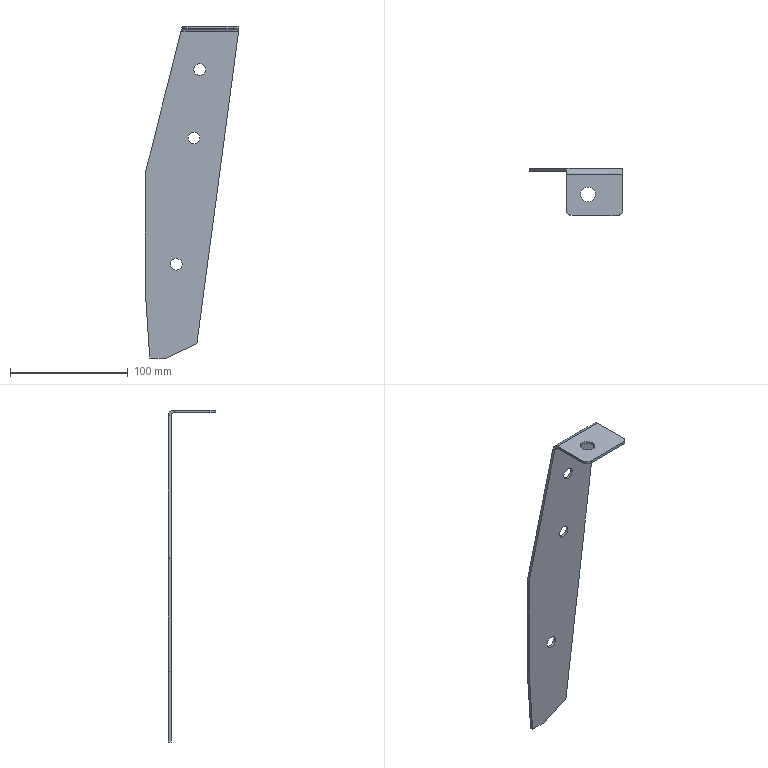Part | SolidWorks | features ICE 2, Fillet 1, FlatPattern 1, SMBaseFlange 1, SheetMetal 1 | 1 solid | 28 faces | box 79.693 x 40 x 281.5 mm | volume 37572 mm3 | cylinder 13 | plane 13 | spline 2 | commonest cylinder face diameters 10 x9 12.5 x2 5 x1 9.6 x1
STEP:
#1=CARTESIAN_POINT('',(3.75,-22.,279.2));
#2=VERTEX_POINT('',#1);
#3=CARTESIAN_POINT('',(16.25,-22.,279.2));
#4=VERTEX_POINT('',#3);
#5=CARTESIAN_POINT('',(10.,-22.,279.2));
#6=DIRECTION('',(0.,0.,1.));
#7=DIRECTION('',(-1.,0.,0.));
#8=AXIS2_PLACEMENT_3D('',#5,#6,#7);
#9=CIRCLE('',#8,6.25);
#10=EDGE_CURVE('',#2,#4,#9,.T.);
#11=ORIENTED_EDGE('',*,*,#10,.F.);
#12=CARTESIAN_POINT('',(3.75,-22.,281.5));
#13=VERTEX_POINT('',#12);
#14=CARTESIAN_POINT('',(3.75,-22.,-0.001));
#15=DIRECTION('',(0.,0.,1.));
#16=VECTOR('',#15,1000.);
#17=LINE('',#14,#16);
#18=EDGE_CURVE('',#2,#13,#17,.T.);
#19=ORIENTED_EDGE('',*,*,#18,.T.);
#20=CARTESIAN_POINT('',(16.25,-22.,281.5));
#21=VERTEX_POINT('',#20);
#22=CARTESIAN_POINT('',(10.,-22.,281.5));
#23=DIRECTION('',(0.,0.,1.));
#24=DIRECTION('',(1.,0.,0.));
#25=AXIS2_PLACEMENT_3D('',#22,#23,#24);
#26=CIRCLE('',#25,6.25);
#27=EDGE_CURVE('',#13,#21,#26,.T.);
#28=ORIENTED_EDGE('',*,*,#27,.T.);
#29=CARTESIAN_POINT('',(16.25,-22.,-0.001));
#30=DIRECTION('',(0.,0.,1.));
#31=VECTOR('',#30,1000.);
#32=LINE('',#29,#31);
#33=EDGE_CURVE('',#4,#21,#32,.T.);
#34=ORIENTED_EDGE('',*,*,#33,.F.);
#35=EDGE_LOOP('',(#11,#19,#28,#34));
#36=FACE_OUTER_BOUND('',#35,.T.);
#37=CARTESIAN_POINT('',(10.,-22.,-0.001));
#38=DIRECTION('',(0.,0.,1.));
#39=DIRECTION('',(1.,0.,0.));
#40=AXIS2_PLACEMENT_3D('',#37,#38,#39);
#41=CYLINDRICAL_SURFACE('',#40,6.25);
#42=ADVANCED_FACE('',(#36),#41,.F.);
#43=CARTESIAN_POINT('',(6.5,0.,249.5));
#44=VERTEX_POINT('',#43);
#45=CARTESIAN_POINT('',(6.5,0.,239.5));
#46=VERTEX_POINT('',#45);
#47=CARTESIAN_POINT('',(6.5,0.,244.5));
#48=DIRECTION('',(0.,-1.,0.));
#49=DIRECTION('',(0.,0.,-1.));
#50=AXIS2_PLACEMENT_3D('',#47,#48,#49);
#51=CIRCLE('',#50,5.);
#52=EDGE_CURVE('',#44,#46,#51,.T.);
#53=ORIENTED_EDGE('',*,*,#52,.F.);
#54=CARTESIAN_POINT('',(6.5,-2.3,249.5));
#55=VERTEX_POINT('',#54);
#56=CARTESIAN_POINT('',(6.5,-2.3,249.5));
#57=DIRECTION('',(0.,-1.,0.));
#58=VECTOR('',#57,1000.);
#59=LINE('',#56,#58);
#60=EDGE_CURVE('',#44,#55,#59,.T.);
#61=ORIENTED_EDGE('',*,*,#60,.T.);
#62=CARTESIAN_POINT('',(6.5,-2.3,239.5));
#63=VERTEX_POINT('',#62);
#64=CARTESIAN_POINT('',(6.5,-2.3,244.5));
#65=DIRECTION('',(0.,-1.,0.));
#66=DIRECTION('',(0.,0.,-1.));
#67=AXIS2_PLACEMENT_3D('',#64,#65,#66);
#68=CIRCLE('',#67,5.);
#69=EDGE_CURVE('',#55,#63,#68,.T.);
#70=ORIENTED_EDGE('',*,*,#69,.T.);
#71=CARTESIAN_POINT('',(6.5,-2.3,239.5));
#72=DIRECTION('',(0.,-1.,0.));
#73=VECTOR('',#72,1000.);
#74=LINE('',#71,#73);
#75=EDGE_CURVE('',#46,#63,#74,.T.);
#76=ORIENTED_EDGE('',*,*,#75,.F.);
#77=EDGE_LOOP('',(#53,#61,#70,#76));
#78=FACE_OUTER_BOUND('',#77,.T.);
#79=CARTESIAN_POINT('',(6.5,-2.3,244.5));
#80=DIRECTION('',(0.,-1.,0.));
#81=DIRECTION('',(0.,0.,-1.));
#82=AXIS2_PLACEMENT_3D('',#79,#80,#81);
#83=CYLINDRICAL_SURFACE('',#82,5.);
#84=ADVANCED_FACE('',(#78),#83,.F.);
#85=CARTESIAN_POINT('',(1.5,0.,191.5));
#86=VERTEX_POINT('',#85);
#87=CARTESIAN_POINT('',(1.5,0.,181.5));
#88=VERTEX_POINT('',#87);
#89=CARTESIAN_POINT('',(1.5,0.,186.5));
#90=DIRECTION('',(0.,-1.,0.));
#91=DIRECTION('',(0.,0.,-1.));
#92=AXIS2_PLACEMENT_3D('',#89,#90,#91);
#93=CIRCLE('',#92,5.);
#94=EDGE_CURVE('',#86,#88,#93,.T.);
#95=ORIENTED_EDGE('',*,*,#94,.F.);
#96=CARTESIAN_POINT('',(1.5,-2.3,191.5));
#97=VERTEX_POINT('',#96);
#98=CARTESIAN_POINT('',(1.5,-2.3,191.5));
#99=DIRECTION('',(0.,-1.,0.));
#100=VECTOR('',#99,1000.);
#101=LINE('',#98,#100);
#102=EDGE_CURVE('',#86,#97,#101,.T.);
#103=ORIENTED_EDGE('',*,*,#102,.T.);
#104=CARTESIAN_POINT('',(1.5,-2.3,181.5));
#105=VERTEX_POINT('',#104);
#106=CARTESIAN_POINT('',(1.5,-2.3,186.5));
#107=DIRECTION('',(0.,-1.,0.));
#108=DIRECTION('',(0.,0.,-1.));
#109=AXIS2_PLACEMENT_3D('',#106,#107,#108);
#110=CIRCLE('',#109,5.);
#111=EDGE_CURVE('',#97,#105,#110,.T.);
#112=ORIENTED_EDGE('',*,*,#111,.T.);
#113=CARTESIAN_POINT('',(1.5,-2.3,181.5));
#114=DIRECTION('',(0.,-1.,0.));
#115=VECTOR('',#114,1000.);
#116=LINE('',#113,#115);
#117=EDGE_CURVE('',#88,#105,#116,.T.);
#118=ORIENTED_EDGE('',*,*,#117,.F.);
#119=EDGE_LOOP('',(#95,#103,#112,#118));
#120=FACE_OUTER_BOUND('',#119,.T.);
#121=CARTESIAN_POINT('',(1.5,-2.3,186.5));
#122=DIRECTION('',(0.,-1.,0.));
#123=DIRECTION('',(0.,0.,-1.));
#124=AXIS2_PLACEMENT_3D('',#121,#122,#123);
#125=CYLINDRICAL_SURFACE('',#124,5.);
#126=ADVANCED_FACE('',(#120),#125,.F.);
#127=CARTESIAN_POINT('',(-13.5,0.,84.5));
#128=VERTEX_POINT('',#127);
#129=CARTESIAN_POINT('',(-13.5,0.,74.5));
#130=VERTEX_POINT('',#129);
#131=CARTESIAN_POINT('',(-13.5,0.,79.5));
#132=DIRECTION('',(0.,-1.,0.));
#133=DIRECTION('',(0.,0.,-1.));
#134=AXIS2_PLACEMENT_3D('',#131,#132,#133);
#135=CIRCLE('',#134,5.);
#136=EDGE_CURVE('',#128,#130,#135,.T.);
#137=ORIENTED_EDGE('',*,*,#136,.F.);
#138=CARTESIAN_POINT('',(-13.5,-2.3,84.5));
#139=VERTEX_POINT('',#138);
#140=CARTESIAN_POINT('',(-13.5,-2.3,84.5));
#141=DIRECTION('',(0.,-1.,0.));
#142=VECTOR('',#141,1000.);
#143=LINE('',#140,#142);
#144=EDGE_CURVE('',#128,#139,#143,.T.);
#145=ORIENTED_EDGE('',*,*,#144,.T.);
#146=CARTESIAN_POINT('',(-13.5,-2.3,74.5));
#147=VERTEX_POINT('',#146);
#148=CARTESIAN_POINT('',(-13.5,-2.3,79.5));
#149=DIRECTION('',(0.,-1.,0.));
#150=DIRECTION('',(0.,0.,-1.));
#151=AXIS2_PLACEMENT_3D('',#148,#149,#150);
#152=CIRCLE('',#151,5.);
#153=EDGE_CURVE('',#139,#147,#152,.T.);
#154=ORIENTED_EDGE('',*,*,#153,.T.);
#155=CARTESIAN_POINT('',(-13.5,-2.3,74.5));
#156=DIRECTION('',(0.,-1.,0.));
#157=VECTOR('',#156,1000.);
#158=LINE('',#155,#157);
#159=EDGE_CURVE('',#130,#147,#158,.T.);
#160=ORIENTED_EDGE('',*,*,#159,.F.);
#161=EDGE_LOOP('',(#137,#145,#154,#160));
#162=FACE_OUTER_BOUND('',#161,.T.);
#163=CARTESIAN_POINT('',(-13.5,-2.3,79.5));
#164=DIRECTION('',(0.,-1.,0.));
#165=DIRECTION('',(0.,0.,-1.));
#166=AXIS2_PLACEMENT_3D('',#163,#164,#165);
#167=CYLINDRICAL_SURFACE('',#166,5.);
#168=ADVANCED_FACE('',(#162),#167,.F.);
#169=CARTESIAN_POINT('',(10.,-22.,281.5));
#170=DIRECTION('',(0.,0.,1.));
#171=DIRECTION('',(1.,0.,0.));
#172=AXIS2_PLACEMENT_3D('',#169,#170,#171);
#173=CIRCLE('',#172,6.25);
#174=EDGE_CURVE('',#21,#13,#173,.T.);
#175=ORIENTED_EDGE('',*,*,#174,.F.);
#176=ORIENTED_EDGE('',*,*,#27,.F.);
#177=EDGE_LOOP('',(#175,#176));
#178=FACE_BOUND('',#177,.T.);
#179=CARTESIAN_POINT('',(34.693,-40.,281.5));
#180=VERTEX_POINT('',#179);
#181=CARTESIAN_POINT('',(-3.3,-40.,281.5));
#182=VERTEX_POINT('',#181);
#183=CARTESIAN_POINT('',(40.,-40.,281.5));
#184=DIRECTION('',(-1.,0.,0.));
#185=VECTOR('',#184,1000.);
#186=LINE('',#183,#185);
#187=EDGE_CURVE('',#180,#182,#186,.T.);
#188=ORIENTED_EDGE('',*,*,#187,.F.);
#189=CARTESIAN_POINT('',(39.693,-35.,281.5));
#190=VERTEX_POINT('',#189);
#191=CARTESIAN_POINT('',(34.693,-35.,281.5));
#192=DIRECTION('',(0.,0.,1.));
#193=DIRECTION('',(-1.,0.,0.));
#194=AXIS2_PLACEMENT_3D('',#191,#192,#193);
#195=CIRCLE('',#194,5.);
#196=EDGE_CURVE('',#180,#190,#195,.T.);
#197=ORIENTED_EDGE('',*,*,#196,.T.);
#198=CARTESIAN_POINT('',(39.693,-4.8,281.5));
#199=VERTEX_POINT('',#198);
#200=CARTESIAN_POINT('',(39.693,0.,281.5));
#201=DIRECTION('',(0.,1.,0.));
#202=VECTOR('',#201,1000.);
#203=LINE('',#200,#202);
#204=EDGE_CURVE('',#190,#199,#203,.T.);
#205=ORIENTED_EDGE('',*,*,#204,.T.);
#206=CARTESIAN_POINT('',(-8.3,-4.8,281.5));
#207=VERTEX_POINT('',#206);
#208=CARTESIAN_POINT('',(40.,-4.8,281.5));
#209=DIRECTION('',(-1.,0.,0.));
#210=VECTOR('',#209,1000.);
#211=LINE('',#208,#210);
#212=EDGE_CURVE('',#199,#207,#211,.T.);
#213=ORIENTED_EDGE('',*,*,#212,.T.);
#214=CARTESIAN_POINT('',(-8.3,-35.,281.5));
#215=VERTEX_POINT('',#214);
#216=CARTESIAN_POINT('',(-8.3,-40.,281.5));
#217=DIRECTION('',(0.,1.,0.));
#218=VECTOR('',#217,1000.);
#219=LINE('',#216,#218);
#220=EDGE_CURVE('',#215,#207,#219,.T.);
#221=ORIENTED_EDGE('',*,*,#220,.F.);
#222=CARTESIAN_POINT('',(-3.3,-35.,281.5));
#223=DIRECTION('',(0.,0.,1.));
#224=DIRECTION('',(-1.,0.,0.));
#225=AXIS2_PLACEMENT_3D('',#222,#223,#224);
#226=CIRCLE('',#225,5.);
#227=EDGE_CURVE('',#215,#182,#226,.T.);
#228=ORIENTED_EDGE('',*,*,#227,.T.);
#229=EDGE_LOOP('',(#188,#197,#205,#213,#221,#228));
#230=FACE_OUTER_BOUND('',#229,.T.);
#231=CARTESIAN_POINT('',(40.,0.,281.5));
#232=DIRECTION('',(0.,0.,-1.));
#233=DIRECTION('',(-1.,0.,0.));
#234=AXIS2_PLACEMENT_3D('',#231,#232,#233);
#235=PLANE('',#234);
#236=ADVANCED_FACE('',(#178,#230),#235,.F.);
#237=CARTESIAN_POINT('',(34.693,-40.,279.2));
#238=VERTEX_POINT('',#237);
#239=CARTESIAN_POINT('',(-3.3,-40.,279.2));
#240=VERTEX_POINT('',#239);
#241=CARTESIAN_POINT('',(40.,-40.,279.2));
#242=DIRECTION('',(-1.,0.,0.));
#243=VECTOR('',#242,1000.);
#244=LINE('',#241,#243);
#245=EDGE_CURVE('',#238,#240,#244,.T.);
#246=ORIENTED_EDGE('',*,*,#245,.F.);
#247=CARTESIAN_POINT('',(34.693,-40.,279.2));
#248=DIRECTION('',(0.,0.,1.));
#249=VECTOR('',#248,1000.);
#250=LINE('',#247,#249);
#251=EDGE_CURVE('',#238,#180,#250,.T.);
#252=ORIENTED_EDGE('',*,*,#251,.T.);
#253=ORIENTED_EDGE('',*,*,#187,.T.);
#254=CARTESIAN_POINT('',(-3.3,-40.,279.2));
#255=DIRECTION('',(0.,0.,-1.));
#256=VECTOR('',#255,1000.);
#257=LINE('',#254,#256);
#258=EDGE_CURVE('',#182,#240,#257,.T.);
#259=ORIENTED_EDGE('',*,*,#258,.T.);
#260=EDGE_LOOP('',(#246,#252,#253,#259));
#261=FACE_OUTER_BOUND('',#260,.T.);
#262=CARTESIAN_POINT('',(40.,-40.,279.2));
#263=DIRECTION('',(0.,-1.,0.));
#264=DIRECTION('',(0.,0.,-1.));
#265=AXIS2_PLACEMENT_3D('',#262,#263,#264);
#266=PLANE('',#265);
#267=ADVANCED_FACE('',(#261),#266,.T.);
#268=CARTESIAN_POINT('',(10.,-22.,279.2));
#269=DIRECTION('',(0.,0.,1.));
#270=DIRECTION('',(-1.,0.,0.));
#271=AXIS2_PLACEMENT_3D('',#268,#269,#270);
#272=CIRCLE('',#271,6.25);
#273=EDGE_CURVE('',#4,#2,#272,.T.);
#274=ORIENTED_EDGE('',*,*,#273,.T.);
#275=ORIENTED_EDGE('',*,*,#10,.T.);
#276=EDGE_LOOP('',(#274,#275));
#277=FACE_BOUND('',#276,.T.);
#278=CARTESIAN_POINT('',(39.693,-35.,279.2));
#279=VERTEX_POINT('',#278);
#280=CARTESIAN_POINT('',(39.693,-4.8,279.2));
#281=VERTEX_POINT('',#280);
#282=CARTESIAN_POINT('',(39.693,0.,279.2));
#283=DIRECTION('',(0.,1.,0.));
#284=VECTOR('',#283,1000.);
#285=LINE('',#282,#284);
#286=EDGE_CURVE('',#279,#281,#285,.T.);
#287=ORIENTED_EDGE('',*,*,#286,.F.);
#288=CARTESIAN_POINT('',(34.693,-35.,279.2));
#289=DIRECTION('',(0.,0.,-1.));
#290=DIRECTION('',(-1.,0.,0.));
#291=AXIS2_PLACEMENT_3D('',#288,#289,#290);
#292=CIRCLE('',#291,5.);
#293=EDGE_CURVE('',#279,#238,#292,.T.);
#294=ORIENTED_EDGE('',*,*,#293,.T.);
#295=ORIENTED_EDGE('',*,*,#245,.T.);
#296=CARTESIAN_POINT('',(-8.3,-35.,279.2));
#297=VERTEX_POINT('',#296);
#298=CARTESIAN_POINT('',(-3.3,-35.,279.2));
#299=DIRECTION('',(0.,0.,-1.));
#300=DIRECTION('',(-1.,0.,0.));
#301=AXIS2_PLACEMENT_3D('',#298,#299,#300);
#302=CIRCLE('',#301,5.);
#303=EDGE_CURVE('',#240,#297,#302,.T.);
#304=ORIENTED_EDGE('',*,*,#303,.T.);
#305=CARTESIAN_POINT('',(-8.3,-4.8,279.2));
#306=VERTEX_POINT('',#305);
#307=CARTESIAN_POINT('',(-8.3,0.,279.2));
#308=DIRECTION('',(0.,1.,0.));
#309=VECTOR('',#308,1000.);
#310=LINE('',#307,#309);
#311=EDGE_CURVE('',#297,#306,#310,.T.);
#312=ORIENTED_EDGE('',*,*,#311,.T.);
#313=CARTESIAN_POINT('',(40.,-4.8,279.2));
#314=DIRECTION('',(-1.,0.,0.));
#315=VECTOR('',#314,1000.);
#316=LINE('',#313,#315);
#317=EDGE_CURVE('',#281,#306,#316,.T.);
#318=ORIENTED_EDGE('',*,*,#317,.F.);
#319=EDGE_LOOP('',(#287,#294,#295,#304,#312,#318));
#320=FACE_OUTER_BOUND('',#319,.T.);
#321=CARTESIAN_POINT('',(40.,0.,279.2));
#322=DIRECTION('',(0.,0.,-1.));
#323=DIRECTION('',(-1.,0.,0.));
#324=AXIS2_PLACEMENT_3D('',#321,#322,#323);
#325=PLANE('',#324);
#326=ADVANCED_FACE('',(#277,#320),#325,.T.);
#327=ORIENTED_EDGE('',*,*,#317,.T.);
#328=CARTESIAN_POINT('',(-9.512,-2.3,276.7));
#329=VERTEX_POINT('',#328);
#330=CARTESIAN_POINT('',(-9.512,-2.3,276.7));
#331=CARTESIAN_POINT('',(-8.802,-2.3,278.164));
#332=CARTESIAN_POINT('',(-8.3,-3.336,279.2));
#333=CARTESIAN_POINT('',(-8.3,-4.8,279.2));
#334=(BOUNDED_CURVE()B_SPLINE_CURVE(3,(#330,#331,#332,#333),.UNSPECIFIED.,.F.,.F.)B_SPLINE_CURVE_WITH_KNOTS((4,4),(1.571,3.142),.UNSPECIFIED.)CURVE()GEOMETRIC_REPRESENTATION_ITEM()RATIONAL_B_SPLINE_CURVE((1.,0.8047,0.8047,1.))REPRESENTATION_ITEM(''));
#335=EDGE_CURVE('',#329,#306,#334,.T.);
#336=ORIENTED_EDGE('',*,*,#335,.F.);
#337=CARTESIAN_POINT('',(39.359,-2.3,276.7));
#338=VERTEX_POINT('',#337);
#339=CARTESIAN_POINT('',(40.,-2.3,276.7));
#340=DIRECTION('',(-1.,0.,0.));
#341=VECTOR('',#340,1000.);
#342=LINE('',#339,#341);
#343=EDGE_CURVE('',#338,#329,#342,.T.);
#344=ORIENTED_EDGE('',*,*,#343,.F.);
#345=CARTESIAN_POINT('',(39.693,-4.8,279.2));
#346=CARTESIAN_POINT('',(39.693,-3.336,279.2));
#347=CARTESIAN_POINT('',(39.554,-2.3,278.164));
#348=CARTESIAN_POINT('',(39.359,-2.3,276.7));
#349=(BOUNDED_CURVE()B_SPLINE_CURVE(3,(#345,#346,#347,#348),.UNSPECIFIED.,.F.,.F.)B_SPLINE_CURVE_WITH_KNOTS((4,4),(3.142,4.712),.UNSPECIFIED.)CURVE()GEOMETRIC_REPRESENTATION_ITEM()RATIONAL_B_SPLINE_CURVE((1.,0.8047,0.8047,1.))REPRESENTATION_ITEM(''));
#350=EDGE_CURVE('',#281,#338,#349,.T.);
#351=ORIENTED_EDGE('',*,*,#350,.F.);
#352=EDGE_LOOP('',(#327,#336,#344,#351));
#353=FACE_OUTER_BOUND('',#352,.T.);
#354=CARTESIAN_POINT('',(40.,-4.8,276.7));
#355=DIRECTION('',(-1.,0.,0.));
#356=DIRECTION('',(0.,0.,1.));
#357=AXIS2_PLACEMENT_3D('',#354,#355,#356);
#358=CYLINDRICAL_SURFACE('',#357,2.5);
#359=ADVANCED_FACE('',(#353),#358,.F.);
#360=CARTESIAN_POINT('',(-22.,-2.3,0.));
#361=VERTEX_POINT('',#360);
#362=CARTESIAN_POINT('',(-36.,-2.3,0.));
#363=VERTEX_POINT('',#362);
#364=CARTESIAN_POINT('',(40.,-2.3,0.));
#365=DIRECTION('',(-1.,0.,0.));
#366=VECTOR('',#365,1000.);
#367=LINE('',#364,#366);
#368=EDGE_CURVE('',#361,#363,#367,.T.);
#369=ORIENTED_EDGE('',*,*,#368,.T.);
#370=CARTESIAN_POINT('',(-36.,0.,0.));
#371=VERTEX_POINT('',#370);
#372=CARTESIAN_POINT('',(-36.,-2.3,0.));
#373=DIRECTION('',(0.,1.,0.));
#374=VECTOR('',#373,1000.);
#375=LINE('',#372,#374);
#376=EDGE_CURVE('',#363,#371,#375,.T.);
#377=ORIENTED_EDGE('',*,*,#376,.T.);
#378=CARTESIAN_POINT('',(-22.,0.,0.));
#379=VERTEX_POINT('',#378);
#380=CARTESIAN_POINT('',(40.,0.,0.));
#381=DIRECTION('',(-1.,0.,0.));
#382=VECTOR('',#381,1000.);
#383=LINE('',#380,#382);
#384=EDGE_CURVE('',#379,#371,#383,.T.);
#385=ORIENTED_EDGE('',*,*,#384,.F.);
#386=CARTESIAN_POINT('',(-22.,0.,0.));
#387=DIRECTION('',(0.,-1.,0.));
#388=VECTOR('',#387,1000.);
#389=LINE('',#386,#388);
#390=EDGE_CURVE('',#379,#361,#389,.T.);
#391=ORIENTED_EDGE('',*,*,#390,.T.);
#392=EDGE_LOOP('',(#369,#377,#385,#391));
#393=FACE_OUTER_BOUND('',#392,.T.);
#394=CARTESIAN_POINT('',(40.,0.,0.));
#395=DIRECTION('',(0.,0.,-1.));
#396=DIRECTION('',(-1.,0.,0.));
#397=AXIS2_PLACEMENT_3D('',#394,#395,#396);
#398=PLANE('',#397);
#399=ADVANCED_FACE('',(#393),#398,.T.);
#400=CARTESIAN_POINT('',(-9.512,0.,276.7));
#401=VERTEX_POINT('',#400);
#402=CARTESIAN_POINT('',(-9.512,0.,276.7));
#403=CARTESIAN_POINT('',(-8.802,0.,279.512));
#404=CARTESIAN_POINT('',(-8.3,-1.988,281.5));
#405=CARTESIAN_POINT('',(-8.3,-4.8,281.5));
#406=(BOUNDED_CURVE()B_SPLINE_CURVE(3,(#402,#403,#404,#405),.UNSPECIFIED.,.F.,.F.)B_SPLINE_CURVE_WITH_KNOTS((4,4),(1.571,3.142),.UNSPECIFIED.)CURVE()GEOMETRIC_REPRESENTATION_ITEM()RATIONAL_B_SPLINE_CURVE((1.,0.8047,0.8047,1.))REPRESENTATION_ITEM(''));
#407=EDGE_CURVE('',#401,#207,#406,.T.);
#408=ORIENTED_EDGE('',*,*,#407,.T.);
#409=ORIENTED_EDGE('',*,*,#212,.F.);
#410=CARTESIAN_POINT('',(39.359,0.,276.7));
#411=VERTEX_POINT('',#410);
#412=CARTESIAN_POINT('',(39.693,-4.8,281.5));
#413=CARTESIAN_POINT('',(39.693,-1.988,281.5));
#414=CARTESIAN_POINT('',(39.554,0.,279.512));
#415=CARTESIAN_POINT('',(39.359,0.,276.7));
#416=(BOUNDED_CURVE()B_SPLINE_CURVE(3,(#412,#413,#414,#415),.UNSPECIFIED.,.F.,.F.)B_SPLINE_CURVE_WITH_KNOTS((4,4),(3.142,4.712),.UNSPECIFIED.)CURVE()GEOMETRIC_REPRESENTATION_ITEM()RATIONAL_B_SPLINE_CURVE((1.,0.8047,0.8047,1.))REPRESENTATION_ITEM(''));
#417=EDGE_CURVE('',#199,#411,#416,.T.);
#418=ORIENTED_EDGE('',*,*,#417,.T.);
#419=CARTESIAN_POINT('',(40.,0.,276.7));
#420=DIRECTION('',(-1.,0.,0.));
#421=VECTOR('',#420,1000.);
#422=LINE('',#419,#421);
#423=EDGE_CURVE('',#411,#401,#422,.T.);
#424=ORIENTED_EDGE('',*,*,#423,.T.);
#425=EDGE_LOOP('',(#408,#409,#418,#424));
#426=FACE_OUTER_BOUND('',#425,.T.);
#427=CARTESIAN_POINT('',(40.,-4.8,276.7));
#428=DIRECTION('',(-1.,0.,0.));
#429=DIRECTION('',(0.,0.,1.));
#430=AXIS2_PLACEMENT_3D('',#427,#428,#429);
#431=CYLINDRICAL_SURFACE('',#430,4.8);
#432=ADVANCED_FACE('',(#426),#431,.T.);
#433=CARTESIAN_POINT('',(-40.,-2.3,60.));
#434=VERTEX_POINT('',#433);
#435=CARTESIAN_POINT('',(-40.,-2.3,155.378));
#436=VERTEX_POINT('',#435);
#437=CARTESIAN_POINT('',(-40.,-2.3,0.));
#438=DIRECTION('',(0.,0.,1.));
#439=VECTOR('',#438,1000.);
#440=LINE('',#437,#439);
#441=EDGE_CURVE('',#434,#436,#440,.T.);
#442=ORIENTED_EDGE('',*,*,#441,.T.);
#443=CARTESIAN_POINT('',(-40.,0.,155.378));
#444=VERTEX_POINT('',#443);
#445=CARTESIAN_POINT('',(-40.,0.,155.378));
#446=DIRECTION('',(0.,1.,0.));
#447=VECTOR('',#446,1000.);
#448=LINE('',#445,#447);
#449=EDGE_CURVE('',#436,#444,#448,.T.);
#450=ORIENTED_EDGE('',*,*,#449,.T.);
#451=CARTESIAN_POINT('',(-40.,0.,60.));
#452=VERTEX_POINT('',#451);
#453=CARTESIAN_POINT('',(-40.,0.,0.));
#454=DIRECTION('',(0.,0.,1.));
#455=VECTOR('',#454,1000.);
#456=LINE('',#453,#455);
#457=EDGE_CURVE('',#452,#444,#456,.T.);
#458=ORIENTED_EDGE('',*,*,#457,.F.);
#459=CARTESIAN_POINT('',(-40.,-2.3,60.));
#460=DIRECTION('',(0.,1.,0.));
#461=VECTOR('',#460,1000.);
#462=LINE('',#459,#461);
#463=EDGE_CURVE('',#434,#452,#462,.T.);
#464=ORIENTED_EDGE('',*,*,#463,.F.);
#465=EDGE_LOOP('',(#442,#450,#458,#464));
#466=FACE_OUTER_BOUND('',#465,.T.);
#467=CARTESIAN_POINT('',(-40.,-4.8,276.7));
#468=DIRECTION('',(1.,0.,0.));
#469=DIRECTION('',(0.,0.,-1.));
#470=AXIS2_PLACEMENT_3D('',#467,#468,#469);
#471=PLANE('',#470);
#472=ADVANCED_FACE('',(#466),#471,.F.);
#473=CARTESIAN_POINT('',(6.5,-2.3,244.5));
#474=DIRECTION('',(0.,-1.,0.));
#475=DIRECTION('',(0.,0.,-1.));
#476=AXIS2_PLACEMENT_3D('',#473,#474,#475);
#477=CIRCLE('',#476,5.);
#478=EDGE_CURVE('',#63,#55,#477,.T.);
#479=ORIENTED_EDGE('',*,*,#478,.F.);
#480=ORIENTED_EDGE('',*,*,#69,.F.);
#481=EDGE_LOOP('',(#479,#480));
#482=FACE_BOUND('',#481,.T.);
#483=CARTESIAN_POINT('',(1.5,-2.3,186.5));
#484=DIRECTION('',(0.,-1.,0.));
#485=DIRECTION('',(0.,0.,-1.));
#486=AXIS2_PLACEMENT_3D('',#483,#484,#485);
#487=CIRCLE('',#486,5.);
#488=EDGE_CURVE('',#105,#97,#487,.T.);
#489=ORIENTED_EDGE('',*,*,#488,.F.);
#490=ORIENTED_EDGE('',*,*,#111,.F.);
#491=EDGE_LOOP('',(#489,#490));
#492=FACE_BOUND('',#491,.T.);
#493=CARTESIAN_POINT('',(-13.5,-2.3,79.5));
#494=DIRECTION('',(0.,-1.,0.));
#495=DIRECTION('',(0.,0.,-1.));
#496=AXIS2_PLACEMENT_3D('',#493,#494,#495);
#497=CIRCLE('',#496,5.);
#498=EDGE_CURVE('',#147,#139,#497,.T.);
#499=ORIENTED_EDGE('',*,*,#498,.F.);
#500=ORIENTED_EDGE('',*,*,#153,.F.);
#501=EDGE_LOOP('',(#499,#500));
#502=FACE_BOUND('',#501,.T.);
#503=CARTESIAN_POINT('',(-39.848,-2.3,156.603));
#504=VERTEX_POINT('',#503);
#505=CARTESIAN_POINT('',(-72.243,-2.3,28.351));
#506=DIRECTION('',(0.2449,0.,0.9695));
#507=VECTOR('',#506,1000.);
#508=LINE('',#505,#507);
#509=EDGE_CURVE('',#504,#329,#508,.T.);
#510=ORIENTED_EDGE('',*,*,#509,.F.);
#511=CARTESIAN_POINT('',(-35.,-2.3,155.378));
#512=DIRECTION('',(0.,-1.,0.));
#513=DIRECTION('',(0.,0.,-1.));
#514=AXIS2_PLACEMENT_3D('',#511,#512,#513);
#515=CIRCLE('',#514,5.);
#516=EDGE_CURVE('',#504,#436,#515,.T.);
#517=ORIENTED_EDGE('',*,*,#516,.T.);
#518=ORIENTED_EDGE('',*,*,#441,.F.);
#519=CARTESIAN_POINT('',(-35.664,-2.3,-5.044));
#520=DIRECTION('',(-0.06652,0.,0.9978));
#521=VECTOR('',#520,1000.);
#522=LINE('',#519,#521);
#523=EDGE_CURVE('',#363,#434,#522,.T.);
#524=ORIENTED_EDGE('',*,*,#523,.F.);
#525=ORIENTED_EDGE('',*,*,#368,.F.);
#526=CARTESIAN_POINT('',(4.,-2.3,12.));
#527=VERTEX_POINT('',#526);
#528=CARTESIAN_POINT('',(4.,-2.3,12.));
#529=DIRECTION('',(0.908,0.,0.4191));
#530=VECTOR('',#529,1000.);
#531=LINE('',#528,#530);
#532=EDGE_CURVE('',#361,#527,#531,.T.);
#533=ORIENTED_EDGE('',*,*,#532,.T.);
#534=CARTESIAN_POINT('',(40.,-2.3,281.5));
#535=DIRECTION('',(0.1324,0.,0.9912));
#536=VECTOR('',#535,1000.);
#537=LINE('',#534,#536);
#538=EDGE_CURVE('',#527,#338,#537,.T.);
#539=ORIENTED_EDGE('',*,*,#538,.T.);
#540=ORIENTED_EDGE('',*,*,#343,.T.);
#541=EDGE_LOOP('',(#510,#517,#518,#524,#525,#533,#539,#540));
#542=FACE_OUTER_BOUND('',#541,.T.);
#543=CARTESIAN_POINT('',(40.,-2.3,0.));
#544=DIRECTION('',(0.,-1.,0.));
#545=DIRECTION('',(0.,0.,-1.));
#546=AXIS2_PLACEMENT_3D('',#543,#544,#545);
#547=PLANE('',#546);
#548=ADVANCED_FACE('',(#482,#492,#502,#542),#547,.T.);
#549=ORIENTED_EDGE('',*,*,#457,.T.);
#550=CARTESIAN_POINT('',(-39.848,0.,156.603));
#551=VERTEX_POINT('',#550);
#552=CARTESIAN_POINT('',(-35.,0.,155.378));
#553=DIRECTION('',(0.,1.,0.));
#554=DIRECTION('',(0.,0.,-1.));
#555=AXIS2_PLACEMENT_3D('',#552,#553,#554);
#556=CIRCLE('',#555,5.);
#557=EDGE_CURVE('',#444,#551,#556,.T.);
#558=ORIENTED_EDGE('',*,*,#557,.T.);
#559=CARTESIAN_POINT('',(-72.243,0.,28.351));
#560=DIRECTION('',(0.2449,0.,0.9695));
#561=VECTOR('',#560,1000.);
#562=LINE('',#559,#561);
#563=EDGE_CURVE('',#551,#401,#562,.T.);
#564=ORIENTED_EDGE('',*,*,#563,.T.);
#565=ORIENTED_EDGE('',*,*,#423,.F.);
#566=CARTESIAN_POINT('',(4.,0.,12.));
#567=VERTEX_POINT('',#566);
#568=CARTESIAN_POINT('',(40.,0.,281.5));
#569=DIRECTION('',(0.1324,0.,0.9912));
#570=VECTOR('',#569,1000.);
#571=LINE('',#568,#570);
#572=EDGE_CURVE('',#567,#411,#571,.T.);
#573=ORIENTED_EDGE('',*,*,#572,.F.);
#574=CARTESIAN_POINT('',(4.,0.,12.));
#575=DIRECTION('',(0.908,0.,0.4191));
#576=VECTOR('',#575,1000.);
#577=LINE('',#574,#576);
#578=EDGE_CURVE('',#379,#567,#577,.T.);
#579=ORIENTED_EDGE('',*,*,#578,.F.);
#580=ORIENTED_EDGE('',*,*,#384,.T.);
#581=CARTESIAN_POINT('',(-35.664,0.,-5.044));
#582=DIRECTION('',(-0.06652,0.,0.9978));
#583=VECTOR('',#582,1000.);
#584=LINE('',#581,#583);
#585=EDGE_CURVE('',#371,#452,#584,.T.);
#586=ORIENTED_EDGE('',*,*,#585,.T.);
#587=EDGE_LOOP('',(#549,#558,#564,#565,#573,#579,#580,#586));
#588=FACE_OUTER_BOUND('',#587,.T.);
#589=CARTESIAN_POINT('',(6.5,0.,244.5));
#590=DIRECTION('',(0.,-1.,0.));
#591=DIRECTION('',(0.,0.,-1.));
#592=AXIS2_PLACEMENT_3D('',#589,#590,#591);
#593=CIRCLE('',#592,5.);
#594=EDGE_CURVE('',#46,#44,#593,.T.);
#595=ORIENTED_EDGE('',*,*,#594,.T.);
#596=ORIENTED_EDGE('',*,*,#52,.T.);
#597=EDGE_LOOP('',(#595,#596));
#598=FACE_BOUND('',#597,.T.);
#599=CARTESIAN_POINT('',(1.5,0.,186.5));
#600=DIRECTION('',(0.,-1.,0.));
#601=DIRECTION('',(0.,0.,-1.));
#602=AXIS2_PLACEMENT_3D('',#599,#600,#601);
#603=CIRCLE('',#602,5.);
#604=EDGE_CURVE('',#88,#86,#603,.T.);
#605=ORIENTED_EDGE('',*,*,#604,.T.);
#606=ORIENTED_EDGE('',*,*,#94,.T.);
#607=EDGE_LOOP('',(#605,#606));
#608=FACE_BOUND('',#607,.T.);
#609=CARTESIAN_POINT('',(-13.5,0.,79.5));
#610=DIRECTION('',(0.,-1.,0.));
#611=DIRECTION('',(0.,0.,-1.));
#612=AXIS2_PLACEMENT_3D('',#609,#610,#611);
#613=CIRCLE('',#612,5.);
#614=EDGE_CURVE('',#130,#128,#613,.T.);
#615=ORIENTED_EDGE('',*,*,#614,.T.);
#616=ORIENTED_EDGE('',*,*,#136,.T.);
#617=EDGE_LOOP('',(#615,#616));
#618=FACE_BOUND('',#617,.T.);
#619=CARTESIAN_POINT('',(40.,0.,0.));
#620=DIRECTION('',(0.,-1.,0.));
#621=DIRECTION('',(0.,0.,-1.));
#622=AXIS2_PLACEMENT_3D('',#619,#620,#621);
#623=PLANE('',#622);
#624=ADVANCED_FACE('',(#588,#598,#608,#618),#623,.F.);
#625=ORIENTED_EDGE('',*,*,#311,.F.);
#626=CARTESIAN_POINT('',(-8.3,-35.,281.5));
#627=DIRECTION('',(0.,0.,1.));
#628=VECTOR('',#627,1000.);
#629=LINE('',#626,#628);
#630=EDGE_CURVE('',#297,#215,#629,.T.);
#631=ORIENTED_EDGE('',*,*,#630,.T.);
#632=ORIENTED_EDGE('',*,*,#220,.T.);
#633=CARTESIAN_POINT('',(-8.3,-4.8,281.5));
#634=DIRECTION('',(0.,0.,-1.));
#635=VECTOR('',#634,1000.);
#636=LINE('',#633,#635);
#637=EDGE_CURVE('',#207,#306,#636,.T.);
#638=ORIENTED_EDGE('',*,*,#637,.T.);
#639=EDGE_LOOP('',(#625,#631,#632,#638));
#640=FACE_OUTER_BOUND('',#639,.T.);
#641=CARTESIAN_POINT('',(-8.3,-40.,281.5));
#642=DIRECTION('',(-1.,0.,0.));
#643=DIRECTION('',(0.,1.,0.));
#644=AXIS2_PLACEMENT_3D('',#641,#642,#643);
#645=PLANE('',#644);
#646=ADVANCED_FACE('',(#640),#645,.T.);
#647=ORIENTED_EDGE('',*,*,#637,.F.);
#648=ORIENTED_EDGE('',*,*,#407,.F.);
#649=CARTESIAN_POINT('',(-9.512,-2.3,276.7));
#650=DIRECTION('',(0.,1.,0.));
#651=VECTOR('',#650,1000.);
#652=LINE('',#649,#651);
#653=EDGE_CURVE('',#329,#401,#652,.T.);
#654=ORIENTED_EDGE('',*,*,#653,.F.);
#655=ORIENTED_EDGE('',*,*,#335,.T.);
#656=EDGE_LOOP('',(#647,#648,#654,#655));
#657=FACE_OUTER_BOUND('',#656,.T.);
#658=CARTESIAN_POINT('',(-10.725,-4.8,274.2));
#659=CARTESIAN_POINT('',(-10.725,-4.8,273.433));
#660=CARTESIAN_POINT('',(-10.725,-4.8,272.667));
#661=CARTESIAN_POINT('',(-10.725,-4.8,271.9));
#662=CARTESIAN_POINT('',(-10.725,0.2,274.2));
#663=CARTESIAN_POINT('',(-10.725,1.733,273.433));
#664=CARTESIAN_POINT('',(-10.725,3.267,272.667));
#665=CARTESIAN_POINT('',(-10.725,4.8,271.9));
#666=CARTESIAN_POINT('',(-8.3,0.2,279.2));
#667=CARTESIAN_POINT('',(-8.3,1.733,279.967));
#668=CARTESIAN_POINT('',(-8.3,3.267,280.733));
#669=CARTESIAN_POINT('',(-8.3,4.8,281.5));
#670=CARTESIAN_POINT('',(-8.3,-4.8,279.2));
#671=CARTESIAN_POINT('',(-8.3,-4.8,279.967));
#672=CARTESIAN_POINT('',(-8.3,-4.8,280.733));
#673=CARTESIAN_POINT('',(-8.3,-4.8,281.5));
#674=CARTESIAN_POINT('',(-8.3,-9.8,279.2));
#675=CARTESIAN_POINT('',(-8.3,-11.333,279.967));
#676=CARTESIAN_POINT('',(-8.3,-12.867,280.733));
#677=CARTESIAN_POINT('',(-8.3,-14.4,281.5));
#678=CARTESIAN_POINT('',(-10.725,-9.8,274.2));
#679=CARTESIAN_POINT('',(-10.725,-11.333,273.433));
#680=CARTESIAN_POINT('',(-10.725,-12.867,272.667));
#681=CARTESIAN_POINT('',(-10.725,-14.4,271.9));
#682=CARTESIAN_POINT('',(-10.725,-4.8,274.2));
#683=CARTESIAN_POINT('',(-10.725,-4.8,273.433));
#684=CARTESIAN_POINT('',(-10.725,-4.8,272.667));
#685=CARTESIAN_POINT('',(-10.725,-4.8,271.9));
#686=(BOUNDED_SURFACE()B_SPLINE_SURFACE(3,3,((#658,#659,#660,#661),(#662,#663,#664,#665),(#666,#667,#668,#669),(#670,#671,#672,#673),(#674,#675,#676,#677),(#678,#679,#680,#681),(#682,#683,#684,#685)),.UNSPECIFIED.,.T.,.F.,.F.)B_SPLINE_SURFACE_WITH_KNOTS((4,3,4),(4,4),(0.,0.5,1.),(0.,1.),.UNSPECIFIED.)GEOMETRIC_REPRESENTATION_ITEM()RATIONAL_B_SPLINE_SURFACE(((1.,1.,1.,1.),(0.3333,0.3333,0.3333,0.3333),(0.3333,0.3333,0.3333,0.3333),(1.,1.,1.,1.),(0.3333,0.3333,0.3333,0.3333),(0.3333,0.3333,0.3333,0.3333),(1.,1.,1.,1.)))REPRESENTATION_ITEM('')SURFACE());
#687=ADVANCED_FACE('',(#657),#686,.T.);
#688=ORIENTED_EDGE('',*,*,#563,.F.);
#689=CARTESIAN_POINT('',(-39.848,-2.3,156.603));
#690=DIRECTION('',(0.,-1.,0.));
#691=VECTOR('',#690,1000.);
#692=LINE('',#689,#691);
#693=EDGE_CURVE('',#551,#504,#692,.T.);
#694=ORIENTED_EDGE('',*,*,#693,.T.);
#695=ORIENTED_EDGE('',*,*,#509,.T.);
#696=ORIENTED_EDGE('',*,*,#653,.T.);
#697=EDGE_LOOP('',(#688,#694,#695,#696));
#698=FACE_OUTER_BOUND('',#697,.T.);
#699=CARTESIAN_POINT('',(-72.243,-2.3,28.351));
#700=DIRECTION('',(0.9695,0.,-0.2449));
#701=DIRECTION('',(0.2449,0.,0.9695));
#702=AXIS2_PLACEMENT_3D('',#699,#700,#701);
#703=PLANE('',#702);
#704=ADVANCED_FACE('',(#698),#703,.F.);
#705=ORIENTED_EDGE('',*,*,#523,.T.);
#706=ORIENTED_EDGE('',*,*,#463,.T.);
#707=ORIENTED_EDGE('',*,*,#585,.F.);
#708=ORIENTED_EDGE('',*,*,#376,.F.);
#709=EDGE_LOOP('',(#705,#706,#707,#708));
#710=FACE_OUTER_BOUND('',#709,.T.);
#711=CARTESIAN_POINT('',(-35.664,-2.3,-5.044));
#712=DIRECTION('',(0.9978,0.,0.06652));
#713=DIRECTION('',(-0.06652,0.,0.9978));
#714=AXIS2_PLACEMENT_3D('',#711,#712,#713);
#715=PLANE('',#714);
#716=ADVANCED_FACE('',(#710),#715,.F.);
#717=ORIENTED_EDGE('',*,*,#390,.F.);
#718=ORIENTED_EDGE('',*,*,#578,.T.);
#719=CARTESIAN_POINT('',(4.,0.,12.));
#720=DIRECTION('',(0.,-1.,0.));
#721=VECTOR('',#720,1000.);
#722=LINE('',#719,#721);
#723=EDGE_CURVE('',#567,#527,#722,.T.);
#724=ORIENTED_EDGE('',*,*,#723,.T.);
#725=ORIENTED_EDGE('',*,*,#532,.F.);
#726=EDGE_LOOP('',(#717,#718,#724,#725));
#727=FACE_OUTER_BOUND('',#726,.T.);
#728=CARTESIAN_POINT('',(4.,0.,12.));
#729=DIRECTION('',(0.4191,0.,-0.908));
#730=DIRECTION('',(0.908,0.,0.4191));
#731=AXIS2_PLACEMENT_3D('',#728,#729,#730);
#732=PLANE('',#731);
#733=ADVANCED_FACE('',(#727),#732,.T.);
#734=ORIENTED_EDGE('',*,*,#723,.F.);
#735=ORIENTED_EDGE('',*,*,#572,.T.);
#736=CARTESIAN_POINT('',(39.359,0.,276.7));
#737=DIRECTION('',(0.,-1.,0.));
#738=VECTOR('',#737,1000.);
#739=LINE('',#736,#738);
#740=EDGE_CURVE('',#411,#338,#739,.T.);
#741=ORIENTED_EDGE('',*,*,#740,.T.);
#742=ORIENTED_EDGE('',*,*,#538,.F.);
#743=EDGE_LOOP('',(#734,#735,#741,#742));
#744=FACE_OUTER_BOUND('',#743,.T.);
#745=CARTESIAN_POINT('',(40.,0.,281.5));
#746=DIRECTION('',(0.9912,0.,-0.1324));
#747=DIRECTION('',(0.1324,0.,0.9912));
#748=AXIS2_PLACEMENT_3D('',#745,#746,#747);
#749=PLANE('',#748);
#750=ADVANCED_FACE('',(#744),#749,.T.);
#751=ORIENTED_EDGE('',*,*,#350,.T.);
#752=ORIENTED_EDGE('',*,*,#740,.F.);
#753=ORIENTED_EDGE('',*,*,#417,.F.);
#754=CARTESIAN_POINT('',(39.693,-4.8,279.2));
#755=DIRECTION('',(0.,0.,1.));
#756=VECTOR('',#755,1000.);
#757=LINE('',#754,#756);
#758=EDGE_CURVE('',#281,#199,#757,.T.);
#759=ORIENTED_EDGE('',*,*,#758,.F.);
#760=EDGE_LOOP('',(#751,#752,#753,#759));
#761=FACE_OUTER_BOUND('',#760,.T.);
#762=CARTESIAN_POINT('',(39.025,-4.8,274.2));
#763=CARTESIAN_POINT('',(39.025,-4.8,273.433));
#764=CARTESIAN_POINT('',(39.025,-4.8,272.667));
#765=CARTESIAN_POINT('',(39.025,-4.8,271.9));
#766=CARTESIAN_POINT('',(39.025,-9.8,274.2));
#767=CARTESIAN_POINT('',(39.025,-11.333,273.433));
#768=CARTESIAN_POINT('',(39.025,-12.867,272.667));
#769=CARTESIAN_POINT('',(39.025,-14.4,271.9));
#770=CARTESIAN_POINT('',(39.693,-9.8,279.2));
#771=CARTESIAN_POINT('',(39.693,-11.333,279.967));
#772=CARTESIAN_POINT('',(39.693,-12.867,280.733));
#773=CARTESIAN_POINT('',(39.693,-14.4,281.5));
#774=CARTESIAN_POINT('',(39.693,-4.8,279.2));
#775=CARTESIAN_POINT('',(39.693,-4.8,279.967));
#776=CARTESIAN_POINT('',(39.693,-4.8,280.733));
#777=CARTESIAN_POINT('',(39.693,-4.8,281.5));
#778=CARTESIAN_POINT('',(39.693,0.2,279.2));
#779=CARTESIAN_POINT('',(39.693,1.733,279.967));
#780=CARTESIAN_POINT('',(39.693,3.267,280.733));
#781=CARTESIAN_POINT('',(39.693,4.8,281.5));
#782=CARTESIAN_POINT('',(39.025,0.2,274.2));
#783=CARTESIAN_POINT('',(39.025,1.733,273.433));
#784=CARTESIAN_POINT('',(39.025,3.267,272.667));
#785=CARTESIAN_POINT('',(39.025,4.8,271.9));
#786=CARTESIAN_POINT('',(39.025,-4.8,274.2));
#787=CARTESIAN_POINT('',(39.025,-4.8,273.433));
#788=CARTESIAN_POINT('',(39.025,-4.8,272.667));
#789=CARTESIAN_POINT('',(39.025,-4.8,271.9));
#790=(BOUNDED_SURFACE()B_SPLINE_SURFACE(3,3,((#762,#763,#764,#765),(#766,#767,#768,#769),(#770,#771,#772,#773),(#774,#775,#776,#777),(#778,#779,#780,#781),(#782,#783,#784,#785),(#786,#787,#788,#789)),.UNSPECIFIED.,.T.,.F.,.T.)B_SPLINE_SURFACE_WITH_KNOTS((4,3,4),(4,4),(0.,0.5,1.),(0.,1.),.UNSPECIFIED.)GEOMETRIC_REPRESENTATION_ITEM()RATIONAL_B_SPLINE_SURFACE(((1.,1.,1.,1.),(0.3333,0.3333,0.3333,0.3333),(0.3333,0.3333,0.3333,0.3333),(1.,1.,1.,1.),(0.3333,0.3333,0.3333,0.3333),(0.3333,0.3333,0.3333,0.3333),(1.,1.,1.,1.)))REPRESENTATION_ITEM('')SURFACE());
#791=ADVANCED_FACE('',(#761),#790,.T.);
#792=ORIENTED_EDGE('',*,*,#204,.F.);
#793=CARTESIAN_POINT('',(39.693,-35.,279.2));
#794=DIRECTION('',(0.,0.,-1.));
#795=VECTOR('',#794,1000.);
#796=LINE('',#793,#795);
#797=EDGE_CURVE('',#190,#279,#796,.T.);
#798=ORIENTED_EDGE('',*,*,#797,.T.);
#799=ORIENTED_EDGE('',*,*,#286,.T.);
#800=ORIENTED_EDGE('',*,*,#758,.T.);
#801=EDGE_LOOP('',(#792,#798,#799,#800));
#802=FACE_OUTER_BOUND('',#801,.T.);
#803=CARTESIAN_POINT('',(39.693,0.,279.2));
#804=DIRECTION('',(-1.,0.,0.));
#805=DIRECTION('',(0.,1.,0.));
#806=AXIS2_PLACEMENT_3D('',#803,#804,#805);
#807=PLANE('',#806);
#808=ADVANCED_FACE('',(#802),#807,.F.);
#809=ORIENTED_EDGE('',*,*,#144,.F.);
#810=ORIENTED_EDGE('',*,*,#614,.F.);
#811=ORIENTED_EDGE('',*,*,#159,.T.);
#812=ORIENTED_EDGE('',*,*,#498,.T.);
#813=EDGE_LOOP('',(#809,#810,#811,#812));
#814=FACE_OUTER_BOUND('',#813,.T.);
#815=CARTESIAN_POINT('',(-13.5,-2.3,79.5));
#816=DIRECTION('',(0.,-1.,0.));
#817=DIRECTION('',(0.,0.,-1.));
#818=AXIS2_PLACEMENT_3D('',#815,#816,#817);
#819=CYLINDRICAL_SURFACE('',#818,5.);
#820=ADVANCED_FACE('',(#814),#819,.F.);
#821=ORIENTED_EDGE('',*,*,#102,.F.);
#822=ORIENTED_EDGE('',*,*,#604,.F.);
#823=ORIENTED_EDGE('',*,*,#117,.T.);
#824=ORIENTED_EDGE('',*,*,#488,.T.);
#825=EDGE_LOOP('',(#821,#822,#823,#824));
#826=FACE_OUTER_BOUND('',#825,.T.);
#827=CARTESIAN_POINT('',(1.5,-2.3,186.5));
#828=DIRECTION('',(0.,-1.,0.));
#829=DIRECTION('',(0.,0.,-1.));
#830=AXIS2_PLACEMENT_3D('',#827,#828,#829);
#831=CYLINDRICAL_SURFACE('',#830,5.);
#832=ADVANCED_FACE('',(#826),#831,.F.);
#833=ORIENTED_EDGE('',*,*,#60,.F.);
#834=ORIENTED_EDGE('',*,*,#594,.F.);
#835=ORIENTED_EDGE('',*,*,#75,.T.);
#836=ORIENTED_EDGE('',*,*,#478,.T.);
#837=EDGE_LOOP('',(#833,#834,#835,#836));
#838=FACE_OUTER_BOUND('',#837,.T.);
#839=CARTESIAN_POINT('',(6.5,-2.3,244.5));
#840=DIRECTION('',(0.,-1.,0.));
#841=DIRECTION('',(0.,0.,-1.));
#842=AXIS2_PLACEMENT_3D('',#839,#840,#841);
#843=CYLINDRICAL_SURFACE('',#842,5.);
#844=ADVANCED_FACE('',(#838),#843,.F.);
#845=ORIENTED_EDGE('',*,*,#18,.F.);
#846=ORIENTED_EDGE('',*,*,#273,.F.);
#847=ORIENTED_EDGE('',*,*,#33,.T.);
#848=ORIENTED_EDGE('',*,*,#174,.T.);
#849=EDGE_LOOP('',(#845,#846,#847,#848));
#850=FACE_OUTER_BOUND('',#849,.T.);
#851=CARTESIAN_POINT('',(10.,-22.,-0.001));
#852=DIRECTION('',(0.,0.,1.));
#853=DIRECTION('',(1.,0.,0.));
#854=AXIS2_PLACEMENT_3D('',#851,#852,#853);
#855=CYLINDRICAL_SURFACE('',#854,6.25);
#856=ADVANCED_FACE('',(#850),#855,.F.);
#857=ORIENTED_EDGE('',*,*,#516,.F.);
#858=ORIENTED_EDGE('',*,*,#693,.F.);
#859=ORIENTED_EDGE('',*,*,#557,.F.);
#860=ORIENTED_EDGE('',*,*,#449,.F.);
#861=EDGE_LOOP('',(#857,#858,#859,#860));
#862=FACE_OUTER_BOUND('',#861,.T.);
#863=CARTESIAN_POINT('',(-35.,-4.8,155.378));
#864=DIRECTION('',(0.,1.,0.));
#865=DIRECTION('',(0.,0.,1.));
#866=AXIS2_PLACEMENT_3D('',#863,#864,#865);
#867=CYLINDRICAL_SURFACE('',#866,5.);
#868=ADVANCED_FACE('',(#862),#867,.T.);
#869=ORIENTED_EDGE('',*,*,#293,.F.);
#870=ORIENTED_EDGE('',*,*,#797,.F.);
#871=ORIENTED_EDGE('',*,*,#196,.F.);
#872=ORIENTED_EDGE('',*,*,#251,.F.);
#873=EDGE_LOOP('',(#869,#870,#871,#872));
#874=FACE_OUTER_BOUND('',#873,.T.);
#875=CARTESIAN_POINT('',(34.693,-35.,279.2));
#876=DIRECTION('',(0.,0.,-1.));
#877=DIRECTION('',(-1.,0.,0.));
#878=AXIS2_PLACEMENT_3D('',#875,#876,#877);
#879=CYLINDRICAL_SURFACE('',#878,5.);
#880=ADVANCED_FACE('',(#874),#879,.T.);
#881=ORIENTED_EDGE('',*,*,#227,.F.);
#882=ORIENTED_EDGE('',*,*,#630,.F.);
#883=ORIENTED_EDGE('',*,*,#303,.F.);
#884=ORIENTED_EDGE('',*,*,#258,.F.);
#885=EDGE_LOOP('',(#881,#882,#883,#884));
#886=FACE_OUTER_BOUND('',#885,.T.);
#887=CARTESIAN_POINT('',(-3.3,-35.,279.2));
#888=DIRECTION('',(0.,0.,-1.));
#889=DIRECTION('',(-1.,0.,0.));
#890=AXIS2_PLACEMENT_3D('',#887,#888,#889);
#891=CYLINDRICAL_SURFACE('',#890,5.);
#892=ADVANCED_FACE('',(#886),#891,.T.);
#893=CLOSED_SHELL('',(#42,#84,#126,#168,#236,#267,#326,#359,#399,#432,#472,#548,#624,#646,#687,#704,#716,#733,#750,#791,#808,#820,#832,#844,#856,#868,#880,#892));
#894=MANIFOLD_SOLID_BREP('',#893);
#895=CARTESIAN_POINT('',(0.,0.,0.));
#896=DIRECTION('',(0.,0.,1.));
#897=DIRECTION('',(1.,0.,0.));
#898=AXIS2_PLACEMENT_3D('',#895,#896,#897);
#899=(LENGTH_UNIT()NAMED_UNIT(*)SI_UNIT(.MILLI.,.METRE.));
#900=UNCERTAINTY_MEASURE_WITH_UNIT(LENGTH_MEASURE(0.00001),#899,'','');
#901=(NAMED_UNIT(*)PLANE_ANGLE_UNIT()SI_UNIT($,.RADIAN.));
#902=(NAMED_UNIT(*)SI_UNIT($,.STERADIAN.)SOLID_ANGLE_UNIT());
#903=(GEOMETRIC_REPRESENTATION_CONTEXT(3)GLOBAL_UNCERTAINTY_ASSIGNED_CONTEXT((#900))GLOBAL_UNIT_ASSIGNED_CONTEXT((#899,#901,#902))REPRESENTATION_CONTEXT('',''));
#904=ADVANCED_BREP_SHAPE_REPRESENTATION('',(#894,#898),#903);